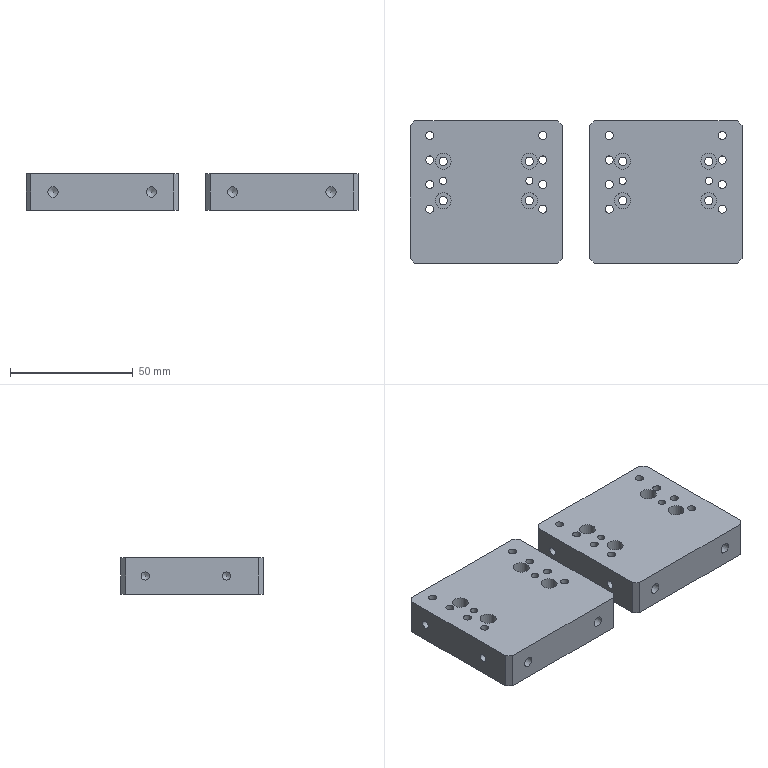Part | 2 solids | 88 faces | box 135 x 58 x 15 mm | volume 100721 mm3 | cylinder 48 | plane 28 | cone 12 | commonest cylinder face diameters 3.3 x24 3.4 x8 6.5 x8 3 x4 4.2 x4